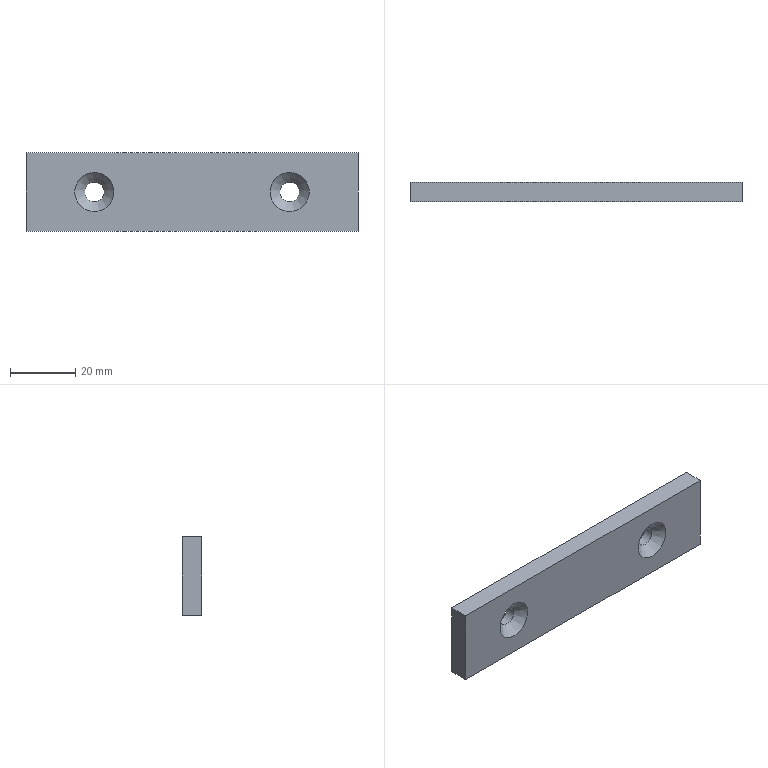Part | NX | features DATUM_CSYS 3, CSUNK_HOLE 2, SKETCH 2, EXTRUDE 1, HOLE PACKAGE 1 | 1 solid | 10 faces | box 102 x 6 x 24 mm | volume 14123 mm3 | plane 6 | cylinder 2 | cone 2 | commonest cylinder face diameters 6 x2
STEP:
#1=CARTESIAN_POINT('',(-51.,0.,12.));
#2=VERTEX_POINT('',#1);
#3=CARTESIAN_POINT('',(-51.,0.,-12.));
#4=VERTEX_POINT('',#3);
#5=CARTESIAN_POINT('',(-51.,0.,12.));
#6=DIRECTION('',(0.,0.,-1.));
#7=VECTOR('',#6,1000.);
#8=LINE('',#5,#7);
#9=EDGE_CURVE('',#2,#4,#8,.T.);
#10=ORIENTED_EDGE('',*,*,#9,.T.);
#11=CARTESIAN_POINT('',(-51.,-6.,-12.));
#12=VERTEX_POINT('',#11);
#13=CARTESIAN_POINT('',(-51.,-6.,-12.));
#14=DIRECTION('',(0.,1.,0.));
#15=VECTOR('',#14,1000.);
#16=LINE('',#13,#15);
#17=EDGE_CURVE('',#12,#4,#16,.T.);
#18=ORIENTED_EDGE('',*,*,#17,.F.);
#19=CARTESIAN_POINT('',(-51.,-6.,12.));
#20=VERTEX_POINT('',#19);
#21=CARTESIAN_POINT('',(-51.,-6.,12.));
#22=DIRECTION('',(0.,0.,-1.));
#23=VECTOR('',#22,1000.);
#24=LINE('',#21,#23);
#25=EDGE_CURVE('',#20,#12,#24,.T.);
#26=ORIENTED_EDGE('',*,*,#25,.F.);
#27=CARTESIAN_POINT('',(-51.,-6.,12.));
#28=DIRECTION('',(0.,1.,0.));
#29=VECTOR('',#28,1000.);
#30=LINE('',#27,#29);
#31=EDGE_CURVE('',#20,#2,#30,.T.);
#32=ORIENTED_EDGE('',*,*,#31,.T.);
#33=EDGE_LOOP('',(#10,#18,#26,#32));
#34=FACE_BOUND('',#33,.T.);
#35=CARTESIAN_POINT('',(-51.,-6.,12.));
#36=DIRECTION('',(1.,0.,0.));
#37=DIRECTION('',(0.,0.,-1.));
#38=AXIS2_PLACEMENT_3D('',#35,#36,#37);
#39=PLANE('',#38);
#40=ADVANCED_FACE('',(#34),#39,.F.);
#41=CARTESIAN_POINT('',(51.,0.,-12.));
#42=VERTEX_POINT('',#41);
#43=CARTESIAN_POINT('',(-51.,0.,-12.));
#44=DIRECTION('',(1.,0.,0.));
#45=VECTOR('',#44,1000.);
#46=LINE('',#43,#45);
#47=EDGE_CURVE('',#4,#42,#46,.T.);
#48=ORIENTED_EDGE('',*,*,#47,.T.);
#49=CARTESIAN_POINT('',(51.,-6.,-12.));
#50=VERTEX_POINT('',#49);
#51=CARTESIAN_POINT('',(51.,-6.,-12.));
#52=DIRECTION('',(0.,1.,0.));
#53=VECTOR('',#52,1000.);
#54=LINE('',#51,#53);
#55=EDGE_CURVE('',#50,#42,#54,.T.);
#56=ORIENTED_EDGE('',*,*,#55,.F.);
#57=CARTESIAN_POINT('',(-51.,-6.,-12.));
#58=DIRECTION('',(1.,0.,0.));
#59=VECTOR('',#58,1000.);
#60=LINE('',#57,#59);
#61=EDGE_CURVE('',#12,#50,#60,.T.);
#62=ORIENTED_EDGE('',*,*,#61,.F.);
#63=ORIENTED_EDGE('',*,*,#17,.T.);
#64=EDGE_LOOP('',(#48,#56,#62,#63));
#65=FACE_BOUND('',#64,.T.);
#66=CARTESIAN_POINT('',(-51.,-6.,-12.));
#67=DIRECTION('',(0.,0.,1.));
#68=DIRECTION('',(1.,0.,0.));
#69=AXIS2_PLACEMENT_3D('',#66,#67,#68);
#70=PLANE('',#69);
#71=ADVANCED_FACE('',(#65),#70,.F.);
#72=CARTESIAN_POINT('',(51.,0.,12.));
#73=VERTEX_POINT('',#72);
#74=CARTESIAN_POINT('',(51.,0.,-12.));
#75=DIRECTION('',(0.,0.,1.));
#76=VECTOR('',#75,1000.);
#77=LINE('',#74,#76);
#78=EDGE_CURVE('',#42,#73,#77,.T.);
#79=ORIENTED_EDGE('',*,*,#78,.T.);
#80=CARTESIAN_POINT('',(51.,-6.,12.));
#81=VERTEX_POINT('',#80);
#82=CARTESIAN_POINT('',(51.,-6.,12.));
#83=DIRECTION('',(0.,1.,0.));
#84=VECTOR('',#83,1000.);
#85=LINE('',#82,#84);
#86=EDGE_CURVE('',#81,#73,#85,.T.);
#87=ORIENTED_EDGE('',*,*,#86,.F.);
#88=CARTESIAN_POINT('',(51.,-6.,-12.));
#89=DIRECTION('',(0.,0.,1.));
#90=VECTOR('',#89,1000.);
#91=LINE('',#88,#90);
#92=EDGE_CURVE('',#50,#81,#91,.T.);
#93=ORIENTED_EDGE('',*,*,#92,.F.);
#94=ORIENTED_EDGE('',*,*,#55,.T.);
#95=EDGE_LOOP('',(#79,#87,#93,#94));
#96=FACE_BOUND('',#95,.T.);
#97=CARTESIAN_POINT('',(51.,-6.,-12.));
#98=DIRECTION('',(-1.,0.,0.));
#99=DIRECTION('',(0.,0.,1.));
#100=AXIS2_PLACEMENT_3D('',#97,#98,#99);
#101=PLANE('',#100);
#102=ADVANCED_FACE('',(#96),#101,.F.);
#103=CARTESIAN_POINT('',(51.,0.,12.));
#104=DIRECTION('',(-1.,0.,0.));
#105=VECTOR('',#104,1000.);
#106=LINE('',#103,#105);
#107=EDGE_CURVE('',#73,#2,#106,.T.);
#108=ORIENTED_EDGE('',*,*,#107,.T.);
#109=ORIENTED_EDGE('',*,*,#31,.F.);
#110=CARTESIAN_POINT('',(51.,-6.,12.));
#111=DIRECTION('',(-1.,0.,0.));
#112=VECTOR('',#111,1000.);
#113=LINE('',#110,#112);
#114=EDGE_CURVE('',#81,#20,#113,.T.);
#115=ORIENTED_EDGE('',*,*,#114,.F.);
#116=ORIENTED_EDGE('',*,*,#86,.T.);
#117=EDGE_LOOP('',(#108,#109,#115,#116));
#118=FACE_BOUND('',#117,.T.);
#119=CARTESIAN_POINT('',(51.,-6.,12.));
#120=DIRECTION('',(0.,0.,-1.));
#121=DIRECTION('',(-1.,0.,0.));
#122=AXIS2_PLACEMENT_3D('',#119,#120,#121);
#123=PLANE('',#122);
#124=ADVANCED_FACE('',(#118),#123,.F.);
#125=CARTESIAN_POINT('',(30.,-6.,6.));
#126=VERTEX_POINT('',#125);
#127=CARTESIAN_POINT('',(30.,-6.,0.));
#128=DIRECTION('',(0.,1.,0.));
#129=DIRECTION('',(0.,0.,1.));
#130=AXIS2_PLACEMENT_3D('',#127,#128,#129);
#131=CIRCLE('',#130,6.);
#132=EDGE_CURVE('',#126,#126,#131,.T.);
#133=ORIENTED_EDGE('',*,*,#132,.T.);
#134=EDGE_LOOP('',(#133));
#135=FACE_BOUND('',#134,.T.);
#136=CARTESIAN_POINT('',(-30.,-6.,6.));
#137=VERTEX_POINT('',#136);
#138=CARTESIAN_POINT('',(-30.,-6.,0.));
#139=DIRECTION('',(0.,1.,0.));
#140=DIRECTION('',(0.,0.,1.));
#141=AXIS2_PLACEMENT_3D('',#138,#139,#140);
#142=CIRCLE('',#141,6.);
#143=EDGE_CURVE('',#137,#137,#142,.T.);
#144=ORIENTED_EDGE('',*,*,#143,.T.);
#145=EDGE_LOOP('',(#144));
#146=FACE_BOUND('',#145,.T.);
#147=ORIENTED_EDGE('',*,*,#25,.T.);
#148=ORIENTED_EDGE('',*,*,#61,.T.);
#149=ORIENTED_EDGE('',*,*,#92,.T.);
#150=ORIENTED_EDGE('',*,*,#114,.T.);
#151=EDGE_LOOP('',(#147,#148,#149,#150));
#152=FACE_BOUND('',#151,.T.);
#153=CARTESIAN_POINT('',(0.,-6.,0.));
#154=DIRECTION('',(0.,-1.,0.));
#155=DIRECTION('',(0.,0.,-1.));
#156=AXIS2_PLACEMENT_3D('',#153,#154,#155);
#157=PLANE('',#156);
#158=ADVANCED_FACE('',(#135,#146,#152),#157,.T.);
#159=CARTESIAN_POINT('',(30.,0.,-3.));
#160=VERTEX_POINT('',#159);
#161=CARTESIAN_POINT('',(30.,0.,0.));
#162=DIRECTION('',(0.,-1.,0.));
#163=DIRECTION('',(0.,0.,-1.));
#164=AXIS2_PLACEMENT_3D('',#161,#162,#163);
#165=CIRCLE('',#164,3.);
#166=EDGE_CURVE('',#160,#160,#165,.T.);
#167=ORIENTED_EDGE('',*,*,#166,.T.);
#168=EDGE_LOOP('',(#167));
#169=FACE_BOUND('',#168,.T.);
#170=CARTESIAN_POINT('',(-30.,0.,-3.));
#171=VERTEX_POINT('',#170);
#172=CARTESIAN_POINT('',(-30.,0.,0.));
#173=DIRECTION('',(0.,-1.,0.));
#174=DIRECTION('',(0.,0.,-1.));
#175=AXIS2_PLACEMENT_3D('',#172,#173,#174);
#176=CIRCLE('',#175,3.);
#177=EDGE_CURVE('',#171,#171,#176,.T.);
#178=ORIENTED_EDGE('',*,*,#177,.T.);
#179=EDGE_LOOP('',(#178));
#180=FACE_BOUND('',#179,.T.);
#181=ORIENTED_EDGE('',*,*,#9,.F.);
#182=ORIENTED_EDGE('',*,*,#107,.F.);
#183=ORIENTED_EDGE('',*,*,#78,.F.);
#184=ORIENTED_EDGE('',*,*,#47,.F.);
#185=EDGE_LOOP('',(#181,#182,#183,#184));
#186=FACE_BOUND('',#185,.T.);
#187=CARTESIAN_POINT('',(0.,0.,0.));
#188=DIRECTION('',(0.,-1.,0.));
#189=DIRECTION('',(0.,0.,-1.));
#190=AXIS2_PLACEMENT_3D('',#187,#188,#189);
#191=PLANE('',#190);
#192=ADVANCED_FACE('',(#169,#180,#186),#191,.F.);
#193=CARTESIAN_POINT('',(-30.,-3.,3.));
#194=VERTEX_POINT('',#193);
#195=CARTESIAN_POINT('',(-30.,-3.,0.));
#196=DIRECTION('',(0.,1.,0.));
#197=DIRECTION('',(0.,0.,1.));
#198=AXIS2_PLACEMENT_3D('',#195,#196,#197);
#199=CIRCLE('',#198,3.);
#200=EDGE_CURVE('',#194,#194,#199,.F.);
#201=ORIENTED_EDGE('',*,*,#200,.T.);
#202=EDGE_LOOP('',(#201));
#203=FACE_BOUND('',#202,.T.);
#204=ORIENTED_EDGE('',*,*,#177,.F.);
#205=EDGE_LOOP('',(#204));
#206=FACE_BOUND('',#205,.T.);
#207=CARTESIAN_POINT('',(-30.,494999.999,0.));
#208=DIRECTION('',(0.,1.,0.));
#209=DIRECTION('',(0.,0.,1.));
#210=AXIS2_PLACEMENT_3D('',#207,#208,#209);
#211=CYLINDRICAL_SURFACE('',#210,3.);
#212=ADVANCED_FACE('',(#203,#206),#211,.F.);
#213=ORIENTED_EDGE('',*,*,#200,.F.);
#214=EDGE_LOOP('',(#213));
#215=FACE_BOUND('',#214,.T.);
#216=ORIENTED_EDGE('',*,*,#143,.F.);
#217=EDGE_LOOP('',(#216));
#218=FACE_BOUND('',#217,.T.);
#219=CARTESIAN_POINT('',(-30.,-6.,0.));
#220=DIRECTION('',(0.,-1.,0.));
#221=DIRECTION('',(0.,0.,-1.));
#222=AXIS2_PLACEMENT_3D('',#219,#220,#221);
#223=CONICAL_SURFACE('',#222,6.,0.7854);
#224=ADVANCED_FACE('',(#215,#218),#223,.F.);
#225=CARTESIAN_POINT('',(30.,-3.,3.));
#226=VERTEX_POINT('',#225);
#227=CARTESIAN_POINT('',(30.,-3.,0.));
#228=DIRECTION('',(0.,1.,0.));
#229=DIRECTION('',(0.,0.,1.));
#230=AXIS2_PLACEMENT_3D('',#227,#228,#229);
#231=CIRCLE('',#230,3.);
#232=EDGE_CURVE('',#226,#226,#231,.F.);
#233=ORIENTED_EDGE('',*,*,#232,.T.);
#234=EDGE_LOOP('',(#233));
#235=FACE_BOUND('',#234,.T.);
#236=ORIENTED_EDGE('',*,*,#166,.F.);
#237=EDGE_LOOP('',(#236));
#238=FACE_BOUND('',#237,.T.);
#239=CARTESIAN_POINT('',(30.,494999.999,0.));
#240=DIRECTION('',(0.,1.,0.));
#241=DIRECTION('',(0.,0.,1.));
#242=AXIS2_PLACEMENT_3D('',#239,#240,#241);
#243=CYLINDRICAL_SURFACE('',#242,3.);
#244=ADVANCED_FACE('',(#235,#238),#243,.F.);
#245=ORIENTED_EDGE('',*,*,#232,.F.);
#246=EDGE_LOOP('',(#245));
#247=FACE_BOUND('',#246,.T.);
#248=ORIENTED_EDGE('',*,*,#132,.F.);
#249=EDGE_LOOP('',(#248));
#250=FACE_BOUND('',#249,.T.);
#251=CARTESIAN_POINT('',(30.,-6.,0.));
#252=DIRECTION('',(0.,-1.,0.));
#253=DIRECTION('',(0.,0.,-1.));
#254=AXIS2_PLACEMENT_3D('',#251,#252,#253);
#255=CONICAL_SURFACE('',#254,6.,0.7854);
#256=ADVANCED_FACE('',(#247,#250),#255,.F.);
#257=CLOSED_SHELL('',(#40,#71,#102,#124,#158,#192,#212,#224,#244,#256));
#258=MANIFOLD_SOLID_BREP('',#257);
#259=(LENGTH_UNIT()NAMED_UNIT(*)SI_UNIT(.MILLI.,.METRE.));
#260=UNCERTAINTY_MEASURE_WITH_UNIT(LENGTH_MEASURE(0.00001),#259,'','');
#261=(NAMED_UNIT(*)PLANE_ANGLE_UNIT()SI_UNIT($,.RADIAN.));
#262=(NAMED_UNIT(*)SI_UNIT($,.STERADIAN.)SOLID_ANGLE_UNIT());
#263=(GEOMETRIC_REPRESENTATION_CONTEXT(3)GLOBAL_UNCERTAINTY_ASSIGNED_CONTEXT((#260))GLOBAL_UNIT_ASSIGNED_CONTEXT((#259,#261,#262))REPRESENTATION_CONTEXT('',''));
#264=ADVANCED_BREP_SHAPE_REPRESENTATION('',(#258),#263);